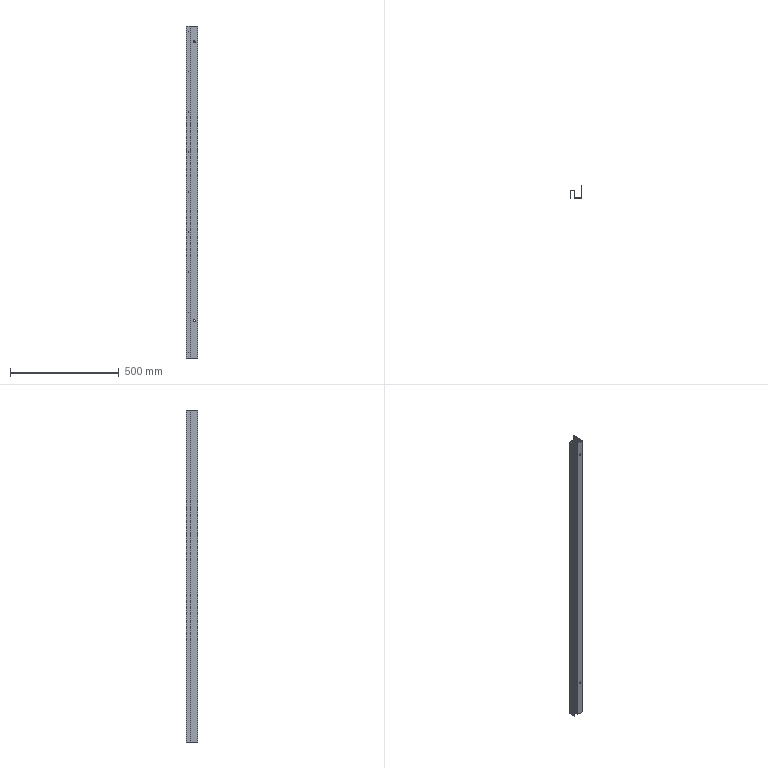Part | STEP file | 1 solid | 36 faces | box 51.2 x 55 x 1530 mm | volume 316686 mm3 | cylinder 22 | plane 14 | commonest cylinder face diameters 3.2 x18 8 x4